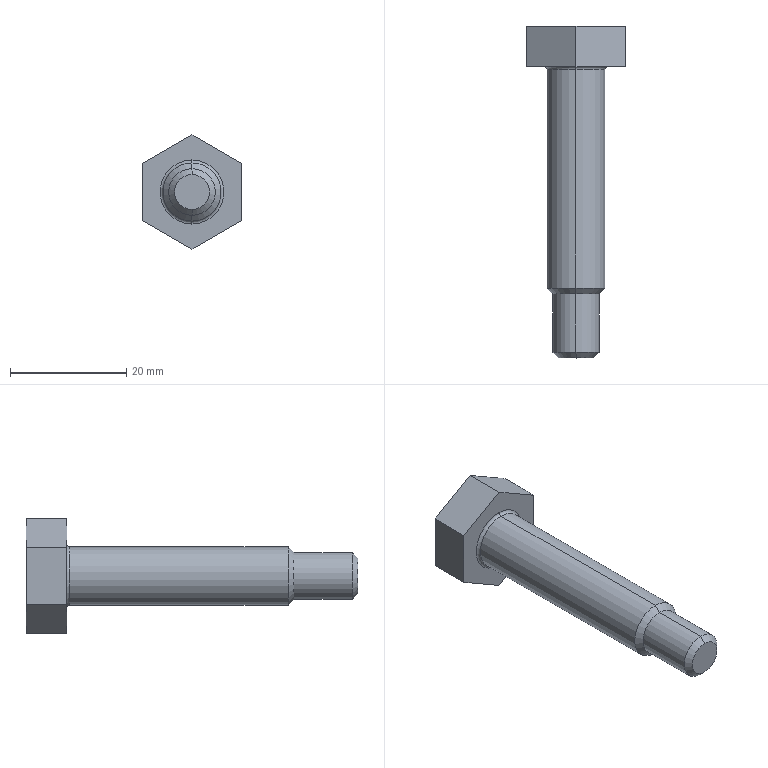Part | SolidWorks | features MirrorStock 1 | 1 solid | 19 faces | box 17 x 57 x 19.63 mm | volume 5343 mm3 | plane 9 | cone 4 | cylinder 4 | torus 2 | commonest cylinder face diameters 8 x2 10 x2
STEP:
#1=CARTESIAN_POINT('',(0.,0.,-5.5));
#2=VERTEX_POINT('',#1);
#3=CARTESIAN_POINT('',(0.,0.,5.5));
#4=VERTEX_POINT('',#3);
#5=CARTESIAN_POINT('',(0.,0.,0.));
#6=DIRECTION('',(0.,-1.,0.));
#7=DIRECTION('',(0.,0.,-1.));
#8=AXIS2_PLACEMENT_3D('',#5,#6,#7);
#9=CIRCLE('',#8,5.5);
#10=EDGE_CURVE('',#2,#4,#9,.T.);
#11=ORIENTED_EDGE('',*,*,#10,.T.);
#12=CARTESIAN_POINT('',(0.,-0.5,5.));
#13=VERTEX_POINT('',#12);
#14=CARTESIAN_POINT('',(0.,-0.5,5.5));
#15=DIRECTION('',(-1.,0.,0.));
#16=DIRECTION('',(0.,0.,1.));
#17=AXIS2_PLACEMENT_3D('',#14,#15,#16);
#18=CIRCLE('',#17,0.5);
#19=EDGE_CURVE('',#4,#13,#18,.T.);
#20=ORIENTED_EDGE('',*,*,#19,.T.);
#21=CARTESIAN_POINT('',(0.,-0.5,-5.));
#22=VERTEX_POINT('',#21);
#23=CARTESIAN_POINT('',(0.,-0.5,0.));
#24=DIRECTION('',(0.,1.,0.));
#25=DIRECTION('',(0.,0.,-1.));
#26=AXIS2_PLACEMENT_3D('',#23,#24,#25);
#27=CIRCLE('',#26,5.);
#28=EDGE_CURVE('',#13,#22,#27,.T.);
#29=ORIENTED_EDGE('',*,*,#28,.T.);
#30=CARTESIAN_POINT('',(0.,-0.5,-5.5));
#31=DIRECTION('',(1.,0.,0.));
#32=DIRECTION('',(0.,0.,-1.));
#33=AXIS2_PLACEMENT_3D('',#30,#31,#32);
#34=CIRCLE('',#33,0.5);
#35=EDGE_CURVE('',#2,#22,#34,.T.);
#36=ORIENTED_EDGE('',*,*,#35,.F.);
#37=EDGE_LOOP('',(#11,#20,#29,#36));
#38=FACE_OUTER_BOUND('',#37,.T.);
#39=CARTESIAN_POINT('',(0.,-0.5,0.));
#40=DIRECTION('',(0.,1.,0.));
#41=DIRECTION('',(0.,0.,-1.));
#42=AXIS2_PLACEMENT_3D('',#39,#40,#41);
#43=TOROIDAL_SURFACE('',#42,5.5,0.5);
#44=ADVANCED_FACE('',(#38),#43,.F.);
#45=CARTESIAN_POINT('',(0.,-50.,-3.));
#46=VERTEX_POINT('',#45);
#47=CARTESIAN_POINT('',(0.,-50.,3.));
#48=VERTEX_POINT('',#47);
#49=CARTESIAN_POINT('',(0.,-50.,0.));
#50=DIRECTION('',(0.,1.,0.));
#51=DIRECTION('',(0.,0.,-1.));
#52=AXIS2_PLACEMENT_3D('',#49,#50,#51);
#53=CIRCLE('',#52,3.);
#54=EDGE_CURVE('',#46,#48,#53,.T.);
#55=ORIENTED_EDGE('',*,*,#54,.T.);
#56=CARTESIAN_POINT('',(0.,-49.,4.));
#57=VERTEX_POINT('',#56);
#58=CARTESIAN_POINT('',(0.,-49.,4.));
#59=DIRECTION('',(0.,0.7071,0.7071));
#60=VECTOR('',#59,1000.);
#61=LINE('',#58,#60);
#62=EDGE_CURVE('',#48,#57,#61,.T.);
#63=ORIENTED_EDGE('',*,*,#62,.T.);
#64=CARTESIAN_POINT('',(0.,-49.,-4.));
#65=VERTEX_POINT('',#64);
#66=CARTESIAN_POINT('',(0.,-49.,0.));
#67=DIRECTION('',(0.,-1.,0.));
#68=DIRECTION('',(0.,0.,-1.));
#69=AXIS2_PLACEMENT_3D('',#66,#67,#68);
#70=CIRCLE('',#69,4.);
#71=EDGE_CURVE('',#57,#65,#70,.T.);
#72=ORIENTED_EDGE('',*,*,#71,.T.);
#73=CARTESIAN_POINT('',(0.,-49.,-4.));
#74=DIRECTION('',(0.,0.7071,-0.7071));
#75=VECTOR('',#74,1000.);
#76=LINE('',#73,#75);
#77=EDGE_CURVE('',#46,#65,#76,.T.);
#78=ORIENTED_EDGE('',*,*,#77,.F.);
#79=EDGE_LOOP('',(#55,#63,#72,#78));
#80=FACE_OUTER_BOUND('',#79,.T.);
#81=CARTESIAN_POINT('',(0.,-49.,0.));
#82=DIRECTION('',(0.,1.,0.));
#83=DIRECTION('',(0.,0.,-1.));
#84=AXIS2_PLACEMENT_3D('',#81,#82,#83);
#85=CONICAL_SURFACE('',#84,4.,0.7854);
#86=ADVANCED_FACE('',(#80),#85,.T.);
#87=CARTESIAN_POINT('',(0.,-38.,5.));
#88=VERTEX_POINT('',#87);
#89=CARTESIAN_POINT('',(0.,-38.,-5.));
#90=VERTEX_POINT('',#89);
#91=CARTESIAN_POINT('',(0.,-38.,0.));
#92=DIRECTION('',(0.,-1.,0.));
#93=DIRECTION('',(0.,0.,-1.));
#94=AXIS2_PLACEMENT_3D('',#91,#92,#93);
#95=CIRCLE('',#94,5.);
#96=EDGE_CURVE('',#88,#90,#95,.T.);
#97=ORIENTED_EDGE('',*,*,#96,.F.);
#98=CARTESIAN_POINT('',(0.,0.,5.));
#99=DIRECTION('',(0.,1.,0.));
#100=VECTOR('',#99,1000.);
#101=LINE('',#98,#100);
#102=EDGE_CURVE('',#88,#13,#101,.T.);
#103=ORIENTED_EDGE('',*,*,#102,.T.);
#104=CARTESIAN_POINT('',(0.,-0.5,0.));
#105=DIRECTION('',(0.,1.,0.));
#106=DIRECTION('',(0.,0.,-1.));
#107=AXIS2_PLACEMENT_3D('',#104,#105,#106);
#108=CIRCLE('',#107,5.);
#109=EDGE_CURVE('',#22,#13,#108,.T.);
#110=ORIENTED_EDGE('',*,*,#109,.F.);
#111=CARTESIAN_POINT('',(0.,0.,-5.));
#112=DIRECTION('',(0.,1.,0.));
#113=VECTOR('',#112,1000.);
#114=LINE('',#111,#113);
#115=EDGE_CURVE('',#90,#22,#114,.T.);
#116=ORIENTED_EDGE('',*,*,#115,.F.);
#117=EDGE_LOOP('',(#97,#103,#110,#116));
#118=FACE_OUTER_BOUND('',#117,.T.);
#119=CARTESIAN_POINT('',(0.,0.,0.));
#120=DIRECTION('',(0.,1.,0.));
#121=DIRECTION('',(0.,0.,-1.));
#122=AXIS2_PLACEMENT_3D('',#119,#120,#121);
#123=CYLINDRICAL_SURFACE('',#122,5.);
#124=ADVANCED_FACE('',(#118),#123,.T.);
#125=CARTESIAN_POINT('',(0.,-39.,4.));
#126=VERTEX_POINT('',#125);
#127=CARTESIAN_POINT('',(0.,-39.,-4.));
#128=VERTEX_POINT('',#127);
#129=CARTESIAN_POINT('',(0.,-39.,0.));
#130=DIRECTION('',(0.,-1.,0.));
#131=DIRECTION('',(0.,0.,-1.));
#132=AXIS2_PLACEMENT_3D('',#129,#130,#131);
#133=CIRCLE('',#132,4.);
#134=EDGE_CURVE('',#126,#128,#133,.T.);
#135=ORIENTED_EDGE('',*,*,#134,.F.);
#136=CARTESIAN_POINT('',(0.,-39.,4.));
#137=DIRECTION('',(0.,0.7071,0.7071));
#138=VECTOR('',#137,1000.);
#139=LINE('',#136,#138);
#140=EDGE_CURVE('',#126,#88,#139,.T.);
#141=ORIENTED_EDGE('',*,*,#140,.T.);
#142=ORIENTED_EDGE('',*,*,#96,.T.);
#143=CARTESIAN_POINT('',(0.,-39.,-4.));
#144=DIRECTION('',(0.,0.7071,-0.7071));
#145=VECTOR('',#144,1000.);
#146=LINE('',#143,#145);
#147=EDGE_CURVE('',#128,#90,#146,.T.);
#148=ORIENTED_EDGE('',*,*,#147,.F.);
#149=EDGE_LOOP('',(#135,#141,#142,#148));
#150=FACE_OUTER_BOUND('',#149,.T.);
#151=CARTESIAN_POINT('',(0.,-39.,0.));
#152=DIRECTION('',(0.,1.,0.));
#153=DIRECTION('',(0.,0.,-1.));
#154=AXIS2_PLACEMENT_3D('',#151,#152,#153);
#155=CONICAL_SURFACE('',#154,4.,0.7854);
#156=ADVANCED_FACE('',(#150),#155,.T.);
#157=ORIENTED_EDGE('',*,*,#71,.F.);
#158=CARTESIAN_POINT('',(0.,0.,4.));
#159=DIRECTION('',(0.,1.,0.));
#160=VECTOR('',#159,1000.);
#161=LINE('',#158,#160);
#162=EDGE_CURVE('',#57,#126,#161,.T.);
#163=ORIENTED_EDGE('',*,*,#162,.T.);
#164=ORIENTED_EDGE('',*,*,#134,.T.);
#165=CARTESIAN_POINT('',(0.,0.,-4.));
#166=DIRECTION('',(0.,1.,0.));
#167=VECTOR('',#166,1000.);
#168=LINE('',#165,#167);
#169=EDGE_CURVE('',#65,#128,#168,.T.);
#170=ORIENTED_EDGE('',*,*,#169,.F.);
#171=EDGE_LOOP('',(#157,#163,#164,#170));
#172=FACE_OUTER_BOUND('',#171,.T.);
#173=CARTESIAN_POINT('',(0.,0.,0.));
#174=DIRECTION('',(0.,1.,0.));
#175=DIRECTION('',(0.,0.,-1.));
#176=AXIS2_PLACEMENT_3D('',#173,#174,#175);
#177=CYLINDRICAL_SURFACE('',#176,4.);
#178=ADVANCED_FACE('',(#172),#177,.T.);
#179=CARTESIAN_POINT('',(8.5,0.,4.907));
#180=VERTEX_POINT('',#179);
#181=CARTESIAN_POINT('',(0.,0.,9.815));
#182=VERTEX_POINT('',#181);
#183=CARTESIAN_POINT('',(8.5,0.,4.907));
#184=DIRECTION('',(-0.866,0.,0.5));
#185=VECTOR('',#184,1000.);
#186=LINE('',#183,#185);
#187=EDGE_CURVE('',#180,#182,#186,.T.);
#188=ORIENTED_EDGE('',*,*,#187,.F.);
#189=CARTESIAN_POINT('',(8.5,7.,4.907));
#190=VERTEX_POINT('',#189);
#191=CARTESIAN_POINT('',(8.5,7.,4.907));
#192=DIRECTION('',(0.,-1.,0.));
#193=VECTOR('',#192,1000.);
#194=LINE('',#191,#193);
#195=EDGE_CURVE('',#190,#180,#194,.T.);
#196=ORIENTED_EDGE('',*,*,#195,.F.);
#197=CARTESIAN_POINT('',(0.,7.,9.815));
#198=VERTEX_POINT('',#197);
#199=CARTESIAN_POINT('',(8.5,7.,4.907));
#200=DIRECTION('',(-0.866,0.,0.5));
#201=VECTOR('',#200,1000.);
#202=LINE('',#199,#201);
#203=EDGE_CURVE('',#190,#198,#202,.T.);
#204=ORIENTED_EDGE('',*,*,#203,.T.);
#205=CARTESIAN_POINT('',(0.,7.,9.815));
#206=DIRECTION('',(0.,-1.,0.));
#207=VECTOR('',#206,1000.);
#208=LINE('',#205,#207);
#209=EDGE_CURVE('',#198,#182,#208,.T.);
#210=ORIENTED_EDGE('',*,*,#209,.T.);
#211=EDGE_LOOP('',(#188,#196,#204,#210));
#212=FACE_OUTER_BOUND('',#211,.T.);
#213=CARTESIAN_POINT('',(8.5,7.,4.907));
#214=DIRECTION('',(-0.5,0.,-0.866));
#215=DIRECTION('',(0.866,0.,-0.5));
#216=AXIS2_PLACEMENT_3D('',#213,#214,#215);
#217=PLANE('',#216);
#218=ADVANCED_FACE('',(#212),#217,.F.);
#219=CARTESIAN_POINT('',(-8.5,0.,4.907));
#220=VERTEX_POINT('',#219);
#221=CARTESIAN_POINT('',(0.,0.,9.815));
#222=DIRECTION('',(-0.866,0.,-0.5));
#223=VECTOR('',#222,1000.);
#224=LINE('',#221,#223);
#225=EDGE_CURVE('',#182,#220,#224,.T.);
#226=ORIENTED_EDGE('',*,*,#225,.F.);
#227=ORIENTED_EDGE('',*,*,#209,.F.);
#228=CARTESIAN_POINT('',(-8.5,7.,4.907));
#229=VERTEX_POINT('',#228);
#230=CARTESIAN_POINT('',(0.,7.,9.815));
#231=DIRECTION('',(-0.866,0.,-0.5));
#232=VECTOR('',#231,1000.);
#233=LINE('',#230,#232);
#234=EDGE_CURVE('',#198,#229,#233,.T.);
#235=ORIENTED_EDGE('',*,*,#234,.T.);
#236=CARTESIAN_POINT('',(-8.5,7.,4.907));
#237=DIRECTION('',(0.,-1.,0.));
#238=VECTOR('',#237,1000.);
#239=LINE('',#236,#238);
#240=EDGE_CURVE('',#229,#220,#239,.T.);
#241=ORIENTED_EDGE('',*,*,#240,.T.);
#242=EDGE_LOOP('',(#226,#227,#235,#241));
#243=FACE_OUTER_BOUND('',#242,.T.);
#244=CARTESIAN_POINT('',(0.,7.,9.815));
#245=DIRECTION('',(0.5,0.,-0.866));
#246=DIRECTION('',(0.866,0.,0.5));
#247=AXIS2_PLACEMENT_3D('',#244,#245,#246);
#248=PLANE('',#247);
#249=ADVANCED_FACE('',(#243),#248,.F.);
#250=CARTESIAN_POINT('',(-8.5,0.,-4.907));
#251=VERTEX_POINT('',#250);
#252=CARTESIAN_POINT('',(-8.5,0.,4.907));
#253=DIRECTION('',(0.,0.,-1.));
#254=VECTOR('',#253,1000.);
#255=LINE('',#252,#254);
#256=EDGE_CURVE('',#220,#251,#255,.T.);
#257=ORIENTED_EDGE('',*,*,#256,.F.);
#258=ORIENTED_EDGE('',*,*,#240,.F.);
#259=CARTESIAN_POINT('',(-8.5,7.,-4.907));
#260=VERTEX_POINT('',#259);
#261=CARTESIAN_POINT('',(-8.5,7.,4.907));
#262=DIRECTION('',(0.,0.,-1.));
#263=VECTOR('',#262,1000.);
#264=LINE('',#261,#263);
#265=EDGE_CURVE('',#229,#260,#264,.T.);
#266=ORIENTED_EDGE('',*,*,#265,.T.);
#267=CARTESIAN_POINT('',(-8.5,7.,-4.907));
#268=DIRECTION('',(0.,-1.,0.));
#269=VECTOR('',#268,1000.);
#270=LINE('',#267,#269);
#271=EDGE_CURVE('',#260,#251,#270,.T.);
#272=ORIENTED_EDGE('',*,*,#271,.T.);
#273=EDGE_LOOP('',(#257,#258,#266,#272));
#274=FACE_OUTER_BOUND('',#273,.T.);
#275=CARTESIAN_POINT('',(-8.5,7.,4.907));
#276=DIRECTION('',(1.,0.,0.));
#277=DIRECTION('',(0.,0.,1.));
#278=AXIS2_PLACEMENT_3D('',#275,#276,#277);
#279=PLANE('',#278);
#280=ADVANCED_FACE('',(#274),#279,.F.);
#281=CARTESIAN_POINT('',(0.,0.,-9.815));
#282=VERTEX_POINT('',#281);
#283=CARTESIAN_POINT('',(-8.5,0.,-4.907));
#284=DIRECTION('',(0.866,0.,-0.5));
#285=VECTOR('',#284,1000.);
#286=LINE('',#283,#285);
#287=EDGE_CURVE('',#251,#282,#286,.T.);
#288=ORIENTED_EDGE('',*,*,#287,.F.);
#289=ORIENTED_EDGE('',*,*,#271,.F.);
#290=CARTESIAN_POINT('',(0.,7.,-9.815));
#291=VERTEX_POINT('',#290);
#292=CARTESIAN_POINT('',(-8.5,7.,-4.907));
#293=DIRECTION('',(0.866,0.,-0.5));
#294=VECTOR('',#293,1000.);
#295=LINE('',#292,#294);
#296=EDGE_CURVE('',#260,#291,#295,.T.);
#297=ORIENTED_EDGE('',*,*,#296,.T.);
#298=CARTESIAN_POINT('',(0.,7.,-9.815));
#299=DIRECTION('',(0.,-1.,0.));
#300=VECTOR('',#299,1000.);
#301=LINE('',#298,#300);
#302=EDGE_CURVE('',#291,#282,#301,.T.);
#303=ORIENTED_EDGE('',*,*,#302,.T.);
#304=EDGE_LOOP('',(#288,#289,#297,#303));
#305=FACE_OUTER_BOUND('',#304,.T.);
#306=CARTESIAN_POINT('',(-8.5,7.,-4.907));
#307=DIRECTION('',(0.5,0.,0.866));
#308=DIRECTION('',(-0.866,0.,0.5));
#309=AXIS2_PLACEMENT_3D('',#306,#307,#308);
#310=PLANE('',#309);
#311=ADVANCED_FACE('',(#305),#310,.F.);
#312=CARTESIAN_POINT('',(8.5,0.,-4.907));
#313=VERTEX_POINT('',#312);
#314=CARTESIAN_POINT('',(0.,0.,-9.815));
#315=DIRECTION('',(0.866,0.,0.5));
#316=VECTOR('',#315,1000.);
#317=LINE('',#314,#316);
#318=EDGE_CURVE('',#282,#313,#317,.T.);
#319=ORIENTED_EDGE('',*,*,#318,.F.);
#320=ORIENTED_EDGE('',*,*,#302,.F.);
#321=CARTESIAN_POINT('',(8.5,7.,-4.907));
#322=VERTEX_POINT('',#321);
#323=CARTESIAN_POINT('',(0.,7.,-9.815));
#324=DIRECTION('',(0.866,0.,0.5));
#325=VECTOR('',#324,1000.);
#326=LINE('',#323,#325);
#327=EDGE_CURVE('',#291,#322,#326,.T.);
#328=ORIENTED_EDGE('',*,*,#327,.T.);
#329=CARTESIAN_POINT('',(8.5,7.,-4.907));
#330=DIRECTION('',(0.,-1.,0.));
#331=VECTOR('',#330,1000.);
#332=LINE('',#329,#331);
#333=EDGE_CURVE('',#322,#313,#332,.T.);
#334=ORIENTED_EDGE('',*,*,#333,.T.);
#335=EDGE_LOOP('',(#319,#320,#328,#334));
#336=FACE_OUTER_BOUND('',#335,.T.);
#337=CARTESIAN_POINT('',(0.,7.,-9.815));
#338=DIRECTION('',(-0.5,0.,0.866));
#339=DIRECTION('',(-0.866,0.,-0.5));
#340=AXIS2_PLACEMENT_3D('',#337,#338,#339);
#341=PLANE('',#340);
#342=ADVANCED_FACE('',(#336),#341,.F.);
#343=CARTESIAN_POINT('',(8.5,0.,-4.907));
#344=DIRECTION('',(0.,0.,1.));
#345=VECTOR('',#344,1000.);
#346=LINE('',#343,#345);
#347=EDGE_CURVE('',#313,#180,#346,.T.);
#348=ORIENTED_EDGE('',*,*,#347,.F.);
#349=ORIENTED_EDGE('',*,*,#333,.F.);
#350=CARTESIAN_POINT('',(8.5,7.,-4.907));
#351=DIRECTION('',(0.,0.,1.));
#352=VECTOR('',#351,1000.);
#353=LINE('',#350,#352);
#354=EDGE_CURVE('',#322,#190,#353,.T.);
#355=ORIENTED_EDGE('',*,*,#354,.T.);
#356=ORIENTED_EDGE('',*,*,#195,.T.);
#357=EDGE_LOOP('',(#348,#349,#355,#356));
#358=FACE_OUTER_BOUND('',#357,.T.);
#359=CARTESIAN_POINT('',(8.5,7.,-4.907));
#360=DIRECTION('',(-1.,0.,0.));
#361=DIRECTION('',(0.,0.,-1.));
#362=AXIS2_PLACEMENT_3D('',#359,#360,#361);
#363=PLANE('',#362);
#364=ADVANCED_FACE('',(#358),#363,.F.);
#365=ORIENTED_EDGE('',*,*,#203,.F.);
#366=ORIENTED_EDGE('',*,*,#354,.F.);
#367=ORIENTED_EDGE('',*,*,#327,.F.);
#368=ORIENTED_EDGE('',*,*,#296,.F.);
#369=ORIENTED_EDGE('',*,*,#265,.F.);
#370=ORIENTED_EDGE('',*,*,#234,.F.);
#371=EDGE_LOOP('',(#365,#366,#367,#368,#369,#370));
#372=FACE_OUTER_BOUND('',#371,.T.);
#373=CARTESIAN_POINT('',(0.,7.,0.));
#374=DIRECTION('',(0.,1.,0.));
#375=DIRECTION('',(0.,0.,-1.));
#376=AXIS2_PLACEMENT_3D('',#373,#374,#375);
#377=PLANE('',#376);
#378=ADVANCED_FACE('',(#372),#377,.T.);
#379=ORIENTED_EDGE('',*,*,#10,.F.);
#380=CARTESIAN_POINT('',(0.,0.,0.));
#381=DIRECTION('',(0.,-1.,0.));
#382=DIRECTION('',(0.,0.,-1.));
#383=AXIS2_PLACEMENT_3D('',#380,#381,#382);
#384=CIRCLE('',#383,5.5);
#385=EDGE_CURVE('',#4,#2,#384,.T.);
#386=ORIENTED_EDGE('',*,*,#385,.F.);
#387=EDGE_LOOP('',(#379,#386));
#388=FACE_BOUND('',#387,.T.);
#389=ORIENTED_EDGE('',*,*,#187,.T.);
#390=ORIENTED_EDGE('',*,*,#225,.T.);
#391=ORIENTED_EDGE('',*,*,#256,.T.);
#392=ORIENTED_EDGE('',*,*,#287,.T.);
#393=ORIENTED_EDGE('',*,*,#318,.T.);
#394=ORIENTED_EDGE('',*,*,#347,.T.);
#395=EDGE_LOOP('',(#389,#390,#391,#392,#393,#394));
#396=FACE_OUTER_BOUND('',#395,.T.);
#397=CARTESIAN_POINT('',(0.,0.,0.));
#398=DIRECTION('',(0.,1.,0.));
#399=DIRECTION('',(0.,0.,-1.));
#400=AXIS2_PLACEMENT_3D('',#397,#398,#399);
#401=PLANE('',#400);
#402=ADVANCED_FACE('',(#388,#396),#401,.F.);
#403=ORIENTED_EDGE('',*,*,#54,.F.);
#404=CARTESIAN_POINT('',(0.,-50.,0.));
#405=DIRECTION('',(0.,1.,0.));
#406=DIRECTION('',(0.,0.,-1.));
#407=AXIS2_PLACEMENT_3D('',#404,#405,#406);
#408=CIRCLE('',#407,3.);
#409=EDGE_CURVE('',#48,#46,#408,.T.);
#410=ORIENTED_EDGE('',*,*,#409,.F.);
#411=EDGE_LOOP('',(#403,#410));
#412=FACE_OUTER_BOUND('',#411,.T.);
#413=CARTESIAN_POINT('',(0.,-50.,0.));
#414=DIRECTION('',(0.,1.,0.));
#415=DIRECTION('',(0.,0.,-1.));
#416=AXIS2_PLACEMENT_3D('',#413,#414,#415);
#417=PLANE('',#416);
#418=ADVANCED_FACE('',(#412),#417,.F.);
#419=ORIENTED_EDGE('',*,*,#162,.F.);
#420=CARTESIAN_POINT('',(0.,-49.,0.));
#421=DIRECTION('',(0.,-1.,0.));
#422=DIRECTION('',(0.,0.,-1.));
#423=AXIS2_PLACEMENT_3D('',#420,#421,#422);
#424=CIRCLE('',#423,4.);
#425=EDGE_CURVE('',#65,#57,#424,.T.);
#426=ORIENTED_EDGE('',*,*,#425,.F.);
#427=ORIENTED_EDGE('',*,*,#169,.T.);
#428=CARTESIAN_POINT('',(0.,-39.,0.));
#429=DIRECTION('',(0.,-1.,0.));
#430=DIRECTION('',(0.,0.,-1.));
#431=AXIS2_PLACEMENT_3D('',#428,#429,#430);
#432=CIRCLE('',#431,4.);
#433=EDGE_CURVE('',#128,#126,#432,.T.);
#434=ORIENTED_EDGE('',*,*,#433,.T.);
#435=EDGE_LOOP('',(#419,#426,#427,#434));
#436=FACE_OUTER_BOUND('',#435,.T.);
#437=CARTESIAN_POINT('',(0.,0.,0.));
#438=DIRECTION('',(0.,1.,0.));
#439=DIRECTION('',(0.,0.,-1.));
#440=AXIS2_PLACEMENT_3D('',#437,#438,#439);
#441=CYLINDRICAL_SURFACE('',#440,4.);
#442=ADVANCED_FACE('',(#436),#441,.T.);
#443=ORIENTED_EDGE('',*,*,#140,.F.);
#444=ORIENTED_EDGE('',*,*,#433,.F.);
#445=ORIENTED_EDGE('',*,*,#147,.T.);
#446=CARTESIAN_POINT('',(0.,-38.,0.));
#447=DIRECTION('',(0.,-1.,0.));
#448=DIRECTION('',(0.,0.,-1.));
#449=AXIS2_PLACEMENT_3D('',#446,#447,#448);
#450=CIRCLE('',#449,5.);
#451=EDGE_CURVE('',#90,#88,#450,.T.);
#452=ORIENTED_EDGE('',*,*,#451,.T.);
#453=EDGE_LOOP('',(#443,#444,#445,#452));
#454=FACE_OUTER_BOUND('',#453,.T.);
#455=CARTESIAN_POINT('',(0.,-39.,0.));
#456=DIRECTION('',(0.,1.,0.));
#457=DIRECTION('',(0.,0.,-1.));
#458=AXIS2_PLACEMENT_3D('',#455,#456,#457);
#459=CONICAL_SURFACE('',#458,4.,0.7854);
#460=ADVANCED_FACE('',(#454),#459,.T.);
#461=ORIENTED_EDGE('',*,*,#102,.F.);
#462=ORIENTED_EDGE('',*,*,#451,.F.);
#463=ORIENTED_EDGE('',*,*,#115,.T.);
#464=ORIENTED_EDGE('',*,*,#28,.F.);
#465=EDGE_LOOP('',(#461,#462,#463,#464));
#466=FACE_OUTER_BOUND('',#465,.T.);
#467=CARTESIAN_POINT('',(0.,0.,0.));
#468=DIRECTION('',(0.,1.,0.));
#469=DIRECTION('',(0.,0.,-1.));
#470=AXIS2_PLACEMENT_3D('',#467,#468,#469);
#471=CYLINDRICAL_SURFACE('',#470,5.);
#472=ADVANCED_FACE('',(#466),#471,.T.);
#473=ORIENTED_EDGE('',*,*,#62,.F.);
#474=ORIENTED_EDGE('',*,*,#409,.T.);
#475=ORIENTED_EDGE('',*,*,#77,.T.);
#476=ORIENTED_EDGE('',*,*,#425,.T.);
#477=EDGE_LOOP('',(#473,#474,#475,#476));
#478=FACE_OUTER_BOUND('',#477,.T.);
#479=CARTESIAN_POINT('',(0.,-49.,0.));
#480=DIRECTION('',(0.,1.,0.));
#481=DIRECTION('',(0.,0.,-1.));
#482=AXIS2_PLACEMENT_3D('',#479,#480,#481);
#483=CONICAL_SURFACE('',#482,4.,0.7854);
#484=ADVANCED_FACE('',(#478),#483,.T.);
#485=ORIENTED_EDGE('',*,*,#19,.F.);
#486=ORIENTED_EDGE('',*,*,#385,.T.);
#487=ORIENTED_EDGE('',*,*,#35,.T.);
#488=ORIENTED_EDGE('',*,*,#109,.T.);
#489=EDGE_LOOP('',(#485,#486,#487,#488));
#490=FACE_OUTER_BOUND('',#489,.T.);
#491=CARTESIAN_POINT('',(0.,-0.5,0.));
#492=DIRECTION('',(0.,1.,0.));
#493=DIRECTION('',(0.,0.,-1.));
#494=AXIS2_PLACEMENT_3D('',#491,#492,#493);
#495=TOROIDAL_SURFACE('',#494,5.5,0.5);
#496=ADVANCED_FACE('',(#490),#495,.F.);
#497=CLOSED_SHELL('',(#44,#86,#124,#156,#178,#218,#249,#280,#311,#342,#364,#378,#402,#418,#442,#460,#472,#484,#496));
#498=MANIFOLD_SOLID_BREP('',#497);
#499=CARTESIAN_POINT('',(0.,0.,0.));
#500=DIRECTION('',(0.,0.,1.));
#501=DIRECTION('',(1.,0.,0.));
#502=AXIS2_PLACEMENT_3D('',#499,#500,#501);
#503=(LENGTH_UNIT()NAMED_UNIT(*)SI_UNIT(.MILLI.,.METRE.));
#504=UNCERTAINTY_MEASURE_WITH_UNIT(LENGTH_MEASURE(0.00001),#503,'','');
#505=(NAMED_UNIT(*)PLANE_ANGLE_UNIT()SI_UNIT($,.RADIAN.));
#506=(NAMED_UNIT(*)SI_UNIT($,.STERADIAN.)SOLID_ANGLE_UNIT());
#507=(GEOMETRIC_REPRESENTATION_CONTEXT(3)GLOBAL_UNCERTAINTY_ASSIGNED_CONTEXT((#504))GLOBAL_UNIT_ASSIGNED_CONTEXT((#503,#505,#506))REPRESENTATION_CONTEXT('',''));
#508=ADVANCED_BREP_SHAPE_REPRESENTATION('',(#498,#502),#507);